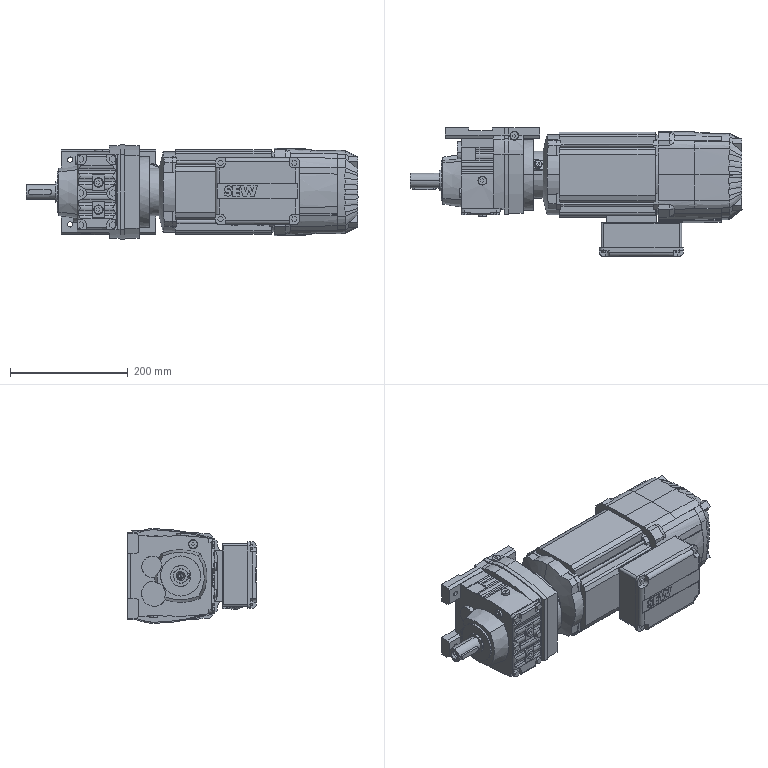Part | SolidWorks | features BaseBody 1 | 1 solid | 913 faces | box 564 x 218.4 x 161 mm | volume 9795428 mm3 | plane 484 | cylinder 291 | spline 76 | cone 62 | commonest cylinder face diameters 0.1 x34 14 x26 22 x23 24 x19 8 x14 16 x12